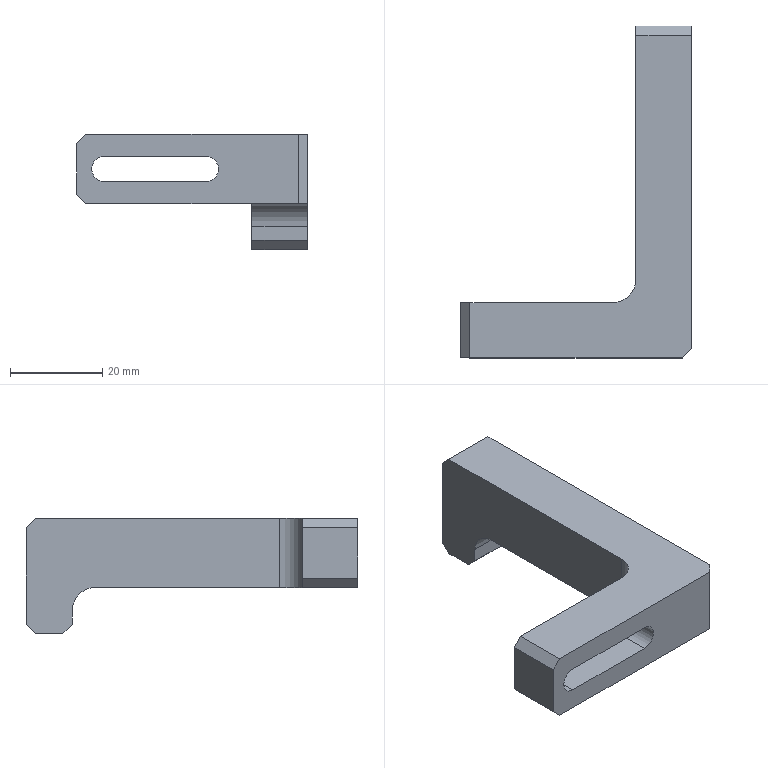Part | NX | 1 solid | 22 faces | box 50 x 72 x 25 mm | volume 19258 mm3 | plane 18 | cylinder 4 | commonest cylinder face diameters 5.5 x2 10 x2
STEP:
#1=CARTESIAN_POINT('',(24.,-33.,-15.));
#2=VERTEX_POINT('',#1);
#3=CARTESIAN_POINT('',(24.,22.,-15.));
#4=VERTEX_POINT('',#3);
#5=CARTESIAN_POINT('',(24.,-35.,-15.));
#6=DIRECTION('',(0.,1.,0.));
#7=VECTOR('',#6,1000.);
#8=LINE('',#5,#7);
#9=EDGE_CURVE('',#2,#4,#8,.T.);
#10=ORIENTED_EDGE('',*,*,#9,.T.);
#11=CARTESIAN_POINT('',(24.,27.,-20.));
#12=VERTEX_POINT('',#11);
#13=CARTESIAN_POINT('',(24.,22.,-20.));
#14=DIRECTION('',(-1.,0.,0.));
#15=DIRECTION('',(0.,0.,-1.));
#16=AXIS2_PLACEMENT_3D('',#13,#14,#15);
#17=CIRCLE('',#16,5.);
#18=EDGE_CURVE('',#4,#12,#17,.T.);
#19=ORIENTED_EDGE('',*,*,#18,.T.);
#20=CARTESIAN_POINT('',(24.,27.,-23.));
#21=VERTEX_POINT('',#20);
#22=CARTESIAN_POINT('',(24.,27.,-15.));
#23=DIRECTION('',(0.,0.,-1.));
#24=VECTOR('',#23,1000.);
#25=LINE('',#22,#24);
#26=EDGE_CURVE('',#12,#21,#25,.T.);
#27=ORIENTED_EDGE('',*,*,#26,.T.);
#28=CARTESIAN_POINT('',(24.,29.,-25.));
#29=VERTEX_POINT('',#28);
#30=CARTESIAN_POINT('',(24.,29.,-25.));
#31=DIRECTION('',(0.,0.7071,-0.7071));
#32=VECTOR('',#31,1000.);
#33=LINE('',#30,#32);
#34=EDGE_CURVE('',#21,#29,#33,.T.);
#35=ORIENTED_EDGE('',*,*,#34,.T.);
#36=CARTESIAN_POINT('',(24.,35.,-25.));
#37=VERTEX_POINT('',#36);
#38=CARTESIAN_POINT('',(24.,-35.,-25.));
#39=DIRECTION('',(0.,1.,0.));
#40=VECTOR('',#39,1000.);
#41=LINE('',#38,#40);
#42=EDGE_CURVE('',#29,#37,#41,.T.);
#43=ORIENTED_EDGE('',*,*,#42,.T.);
#44=CARTESIAN_POINT('',(24.,37.,-23.));
#45=VERTEX_POINT('',#44);
#46=CARTESIAN_POINT('',(24.,35.,-25.));
#47=DIRECTION('',(0.,0.7071,0.7071));
#48=VECTOR('',#47,1000.);
#49=LINE('',#46,#48);
#50=EDGE_CURVE('',#37,#45,#49,.T.);
#51=ORIENTED_EDGE('',*,*,#50,.T.);
#52=CARTESIAN_POINT('',(24.,37.,-2.));
#53=VERTEX_POINT('',#52);
#54=CARTESIAN_POINT('',(24.,37.,-25.));
#55=DIRECTION('',(0.,0.,1.));
#56=VECTOR('',#55,1000.);
#57=LINE('',#54,#56);
#58=EDGE_CURVE('',#45,#53,#57,.T.);
#59=ORIENTED_EDGE('',*,*,#58,.T.);
#60=CARTESIAN_POINT('',(24.,35.,0.));
#61=VERTEX_POINT('',#60);
#62=CARTESIAN_POINT('',(24.,35.,0.));
#63=DIRECTION('',(0.,-0.7071,0.7071));
#64=VECTOR('',#63,1000.);
#65=LINE('',#62,#64);
#66=EDGE_CURVE('',#53,#61,#65,.T.);
#67=ORIENTED_EDGE('',*,*,#66,.T.);
#68=CARTESIAN_POINT('',(24.,-33.,0.));
#69=VERTEX_POINT('',#68);
#70=CARTESIAN_POINT('',(24.,-35.,0.));
#71=DIRECTION('',(0.,1.,0.));
#72=VECTOR('',#71,1000.);
#73=LINE('',#70,#72);
#74=EDGE_CURVE('',#69,#61,#73,.T.);
#75=ORIENTED_EDGE('',*,*,#74,.F.);
#76=CARTESIAN_POINT('',(24.,-33.,-25.));
#77=DIRECTION('',(0.,0.,-1.));
#78=VECTOR('',#77,1000.);
#79=LINE('',#76,#78);
#80=EDGE_CURVE('',#69,#2,#79,.T.);
#81=ORIENTED_EDGE('',*,*,#80,.T.);
#82=EDGE_LOOP('',(#10,#19,#27,#35,#43,#51,#59,#67,#75,#81));
#83=FACE_BOUND('',#82,.T.);
#84=CARTESIAN_POINT('',(24.,-35.,-25.));
#85=DIRECTION('',(-1.,0.,0.));
#86=DIRECTION('',(0.,0.,1.));
#87=AXIS2_PLACEMENT_3D('',#84,#85,#86);
#88=PLANE('',#87);
#89=ADVANCED_FACE('',(#83),#88,.F.);
#90=ORIENTED_EDGE('',*,*,#74,.T.);
#91=CARTESIAN_POINT('',(12.,35.,0.));
#92=VERTEX_POINT('',#91);
#93=CARTESIAN_POINT('',(12.,35.,0.));
#94=DIRECTION('',(-1.,0.,0.));
#95=VECTOR('',#94,1000.);
#96=LINE('',#93,#95);
#97=EDGE_CURVE('',#61,#92,#96,.T.);
#98=ORIENTED_EDGE('',*,*,#97,.T.);
#99=CARTESIAN_POINT('',(12.,-18.,0.));
#100=VERTEX_POINT('',#99);
#101=CARTESIAN_POINT('',(12.,-23.,0.));
#102=DIRECTION('',(0.,1.,0.));
#103=VECTOR('',#102,1000.);
#104=LINE('',#101,#103);
#105=EDGE_CURVE('',#100,#92,#104,.T.);
#106=ORIENTED_EDGE('',*,*,#105,.F.);
#107=CARTESIAN_POINT('',(7.,-23.,0.));
#108=VERTEX_POINT('',#107);
#109=CARTESIAN_POINT('',(7.,-18.,0.));
#110=DIRECTION('',(0.,0.,-1.));
#111=DIRECTION('',(1.,0.,0.));
#112=AXIS2_PLACEMENT_3D('',#109,#110,#111);
#113=CIRCLE('',#112,5.);
#114=EDGE_CURVE('',#100,#108,#113,.T.);
#115=ORIENTED_EDGE('',*,*,#114,.T.);
#116=CARTESIAN_POINT('',(-24.,-23.,0.));
#117=VERTEX_POINT('',#116);
#118=CARTESIAN_POINT('',(-26.,-23.,0.));
#119=DIRECTION('',(1.,0.,0.));
#120=VECTOR('',#119,1000.);
#121=LINE('',#118,#120);
#122=EDGE_CURVE('',#117,#108,#121,.T.);
#123=ORIENTED_EDGE('',*,*,#122,.F.);
#124=CARTESIAN_POINT('',(-24.,-35.,0.));
#125=VERTEX_POINT('',#124);
#126=CARTESIAN_POINT('',(-24.,-35.,0.));
#127=DIRECTION('',(0.,-1.,0.));
#128=VECTOR('',#127,1000.);
#129=LINE('',#126,#128);
#130=EDGE_CURVE('',#117,#125,#129,.T.);
#131=ORIENTED_EDGE('',*,*,#130,.T.);
#132=CARTESIAN_POINT('',(22.,-35.,0.));
#133=VERTEX_POINT('',#132);
#134=CARTESIAN_POINT('',(-26.,-35.,0.));
#135=DIRECTION('',(-1.,0.,0.));
#136=VECTOR('',#135,1000.);
#137=LINE('',#134,#136);
#138=EDGE_CURVE('',#133,#125,#137,.T.);
#139=ORIENTED_EDGE('',*,*,#138,.F.);
#140=CARTESIAN_POINT('',(22.,-35.,0.));
#141=DIRECTION('',(0.7071,0.7071,0.));
#142=VECTOR('',#141,1000.);
#143=LINE('',#140,#142);
#144=EDGE_CURVE('',#133,#69,#143,.T.);
#145=ORIENTED_EDGE('',*,*,#144,.T.);
#146=EDGE_LOOP('',(#90,#98,#106,#115,#123,#131,#139,#145));
#147=FACE_BOUND('',#146,.T.);
#148=CARTESIAN_POINT('',(-26.,-35.,0.));
#149=DIRECTION('',(0.,0.,-1.));
#150=DIRECTION('',(-1.,0.,0.));
#151=AXIS2_PLACEMENT_3D('',#148,#149,#150);
#152=PLANE('',#151);
#153=ADVANCED_FACE('',(#147),#152,.F.);
#154=CARTESIAN_POINT('',(-26.,-35.,-2.));
#155=VERTEX_POINT('',#154);
#156=CARTESIAN_POINT('',(-26.,-35.,-13.));
#157=VERTEX_POINT('',#156);
#158=CARTESIAN_POINT('',(-26.,-35.,-25.));
#159=DIRECTION('',(0.,0.,-1.));
#160=VECTOR('',#159,1000.);
#161=LINE('',#158,#160);
#162=EDGE_CURVE('',#155,#157,#161,.T.);
#163=ORIENTED_EDGE('',*,*,#162,.F.);
#164=CARTESIAN_POINT('',(-26.,-23.,-2.));
#165=VERTEX_POINT('',#164);
#166=CARTESIAN_POINT('',(-26.,-35.,-2.));
#167=DIRECTION('',(0.,1.,0.));
#168=VECTOR('',#167,1000.);
#169=LINE('',#166,#168);
#170=EDGE_CURVE('',#155,#165,#169,.T.);
#171=ORIENTED_EDGE('',*,*,#170,.T.);
#172=CARTESIAN_POINT('',(-26.,-23.,-13.));
#173=VERTEX_POINT('',#172);
#174=CARTESIAN_POINT('',(-26.,-23.,-25.));
#175=DIRECTION('',(0.,0.,1.));
#176=VECTOR('',#175,1000.);
#177=LINE('',#174,#176);
#178=EDGE_CURVE('',#173,#165,#177,.T.);
#179=ORIENTED_EDGE('',*,*,#178,.F.);
#180=CARTESIAN_POINT('',(-26.,-35.,-13.));
#181=DIRECTION('',(0.,-1.,0.));
#182=VECTOR('',#181,1000.);
#183=LINE('',#180,#182);
#184=EDGE_CURVE('',#173,#157,#183,.T.);
#185=ORIENTED_EDGE('',*,*,#184,.T.);
#186=EDGE_LOOP('',(#163,#171,#179,#185));
#187=FACE_BOUND('',#186,.T.);
#188=CARTESIAN_POINT('',(-26.,-35.,-25.));
#189=DIRECTION('',(1.,0.,0.));
#190=DIRECTION('',(0.,1.,0.));
#191=AXIS2_PLACEMENT_3D('',#188,#189,#190);
#192=PLANE('',#191);
#193=ADVANCED_FACE('',(#187),#192,.F.);
#194=ORIENTED_EDGE('',*,*,#42,.F.);
#195=CARTESIAN_POINT('',(12.,29.,-25.));
#196=VERTEX_POINT('',#195);
#197=CARTESIAN_POINT('',(-26.,29.,-25.));
#198=DIRECTION('',(-1.,0.,0.));
#199=VECTOR('',#198,1000.);
#200=LINE('',#197,#199);
#201=EDGE_CURVE('',#29,#196,#200,.T.);
#202=ORIENTED_EDGE('',*,*,#201,.T.);
#203=CARTESIAN_POINT('',(12.,35.,-25.));
#204=VERTEX_POINT('',#203);
#205=CARTESIAN_POINT('',(12.,-23.,-25.));
#206=DIRECTION('',(0.,1.,0.));
#207=VECTOR('',#206,1000.);
#208=LINE('',#205,#207);
#209=EDGE_CURVE('',#196,#204,#208,.T.);
#210=ORIENTED_EDGE('',*,*,#209,.T.);
#211=CARTESIAN_POINT('',(24.,35.,-25.));
#212=DIRECTION('',(1.,0.,0.));
#213=VECTOR('',#212,1000.);
#214=LINE('',#211,#213);
#215=EDGE_CURVE('',#204,#37,#214,.T.);
#216=ORIENTED_EDGE('',*,*,#215,.T.);
#217=EDGE_LOOP('',(#194,#202,#210,#216));
#218=FACE_BOUND('',#217,.T.);
#219=CARTESIAN_POINT('',(-26.,-35.,-25.));
#220=DIRECTION('',(0.,0.,1.));
#221=DIRECTION('',(1.,0.,0.));
#222=AXIS2_PLACEMENT_3D('',#219,#220,#221);
#223=PLANE('',#222);
#224=ADVANCED_FACE('',(#218),#223,.F.);
#225=CARTESIAN_POINT('',(-20.,-35.,-4.75));
#226=VERTEX_POINT('',#225);
#227=CARTESIAN_POINT('',(2.,-35.,-4.75));
#228=VERTEX_POINT('',#227);
#229=CARTESIAN_POINT('',(-20.,-35.,-4.75));
#230=DIRECTION('',(1.,0.,0.));
#231=VECTOR('',#230,1000.);
#232=LINE('',#229,#231);
#233=EDGE_CURVE('',#226,#228,#232,.T.);
#234=ORIENTED_EDGE('',*,*,#233,.T.);
#235=CARTESIAN_POINT('',(2.,-35.,-10.25));
#236=VERTEX_POINT('',#235);
#237=CARTESIAN_POINT('',(2.,-35.,-7.5));
#238=DIRECTION('',(0.,1.,0.));
#239=DIRECTION('',(0.,0.,-1.));
#240=AXIS2_PLACEMENT_3D('',#237,#238,#239);
#241=CIRCLE('',#240,2.75);
#242=EDGE_CURVE('',#228,#236,#241,.T.);
#243=ORIENTED_EDGE('',*,*,#242,.T.);
#244=CARTESIAN_POINT('',(-20.,-35.,-10.25));
#245=VERTEX_POINT('',#244);
#246=CARTESIAN_POINT('',(-20.,-35.,-10.25));
#247=DIRECTION('',(1.,0.,0.));
#248=VECTOR('',#247,1000.);
#249=LINE('',#246,#248);
#250=EDGE_CURVE('',#245,#236,#249,.T.);
#251=ORIENTED_EDGE('',*,*,#250,.F.);
#252=CARTESIAN_POINT('',(-20.,-35.,-7.5));
#253=DIRECTION('',(0.,1.,0.));
#254=DIRECTION('',(0.,0.,-1.));
#255=AXIS2_PLACEMENT_3D('',#252,#253,#254);
#256=CIRCLE('',#255,2.75);
#257=EDGE_CURVE('',#245,#226,#256,.T.);
#258=ORIENTED_EDGE('',*,*,#257,.T.);
#259=EDGE_LOOP('',(#234,#243,#251,#258));
#260=FACE_BOUND('',#259,.T.);
#261=CARTESIAN_POINT('',(22.,-35.,-15.));
#262=VERTEX_POINT('',#261);
#263=CARTESIAN_POINT('',(-24.,-35.,-15.));
#264=VERTEX_POINT('',#263);
#265=CARTESIAN_POINT('',(24.,-35.,-15.));
#266=DIRECTION('',(-1.,0.,0.));
#267=VECTOR('',#266,1000.);
#268=LINE('',#265,#267);
#269=EDGE_CURVE('',#262,#264,#268,.T.);
#270=ORIENTED_EDGE('',*,*,#269,.F.);
#271=CARTESIAN_POINT('',(22.,-35.,-12.5));
#272=DIRECTION('',(0.,0.,1.));
#273=VECTOR('',#272,1000.);
#274=LINE('',#271,#273);
#275=EDGE_CURVE('',#262,#133,#274,.T.);
#276=ORIENTED_EDGE('',*,*,#275,.T.);
#277=ORIENTED_EDGE('',*,*,#138,.T.);
#278=CARTESIAN_POINT('',(-26.,-35.,-2.));
#279=DIRECTION('',(-0.7071,0.,-0.7071));
#280=VECTOR('',#279,1000.);
#281=LINE('',#278,#280);
#282=EDGE_CURVE('',#125,#155,#281,.T.);
#283=ORIENTED_EDGE('',*,*,#282,.T.);
#284=ORIENTED_EDGE('',*,*,#162,.T.);
#285=CARTESIAN_POINT('',(-24.,-35.,-15.));
#286=DIRECTION('',(0.7071,0.,-0.7071));
#287=VECTOR('',#286,1000.);
#288=LINE('',#285,#287);
#289=EDGE_CURVE('',#157,#264,#288,.T.);
#290=ORIENTED_EDGE('',*,*,#289,.T.);
#291=EDGE_LOOP('',(#270,#276,#277,#283,#284,#290));
#292=FACE_BOUND('',#291,.T.);
#293=CARTESIAN_POINT('',(-1.,-35.,-12.5));
#294=DIRECTION('',(0.,1.,0.));
#295=DIRECTION('',(-1.,0.,0.));
#296=AXIS2_PLACEMENT_3D('',#293,#294,#295);
#297=PLANE('',#296);
#298=ADVANCED_FACE('',(#260,#292),#297,.F.);
#299=ORIENTED_EDGE('',*,*,#58,.F.);
#300=CARTESIAN_POINT('',(12.,37.,-23.));
#301=VERTEX_POINT('',#300);
#302=CARTESIAN_POINT('',(12.,37.,-23.));
#303=DIRECTION('',(-1.,0.,0.));
#304=VECTOR('',#303,1000.);
#305=LINE('',#302,#304);
#306=EDGE_CURVE('',#45,#301,#305,.T.);
#307=ORIENTED_EDGE('',*,*,#306,.T.);
#308=CARTESIAN_POINT('',(12.,37.,-2.));
#309=VERTEX_POINT('',#308);
#310=CARTESIAN_POINT('',(12.,37.,-25.));
#311=DIRECTION('',(0.,0.,1.));
#312=VECTOR('',#311,1000.);
#313=LINE('',#310,#312);
#314=EDGE_CURVE('',#301,#309,#313,.T.);
#315=ORIENTED_EDGE('',*,*,#314,.T.);
#316=CARTESIAN_POINT('',(24.,37.,-2.));
#317=DIRECTION('',(1.,0.,0.));
#318=VECTOR('',#317,1000.);
#319=LINE('',#316,#318);
#320=EDGE_CURVE('',#309,#53,#319,.T.);
#321=ORIENTED_EDGE('',*,*,#320,.T.);
#322=EDGE_LOOP('',(#299,#307,#315,#321));
#323=FACE_BOUND('',#322,.T.);
#324=CARTESIAN_POINT('',(-1.,37.,-12.5));
#325=DIRECTION('',(0.,1.,0.));
#326=DIRECTION('',(-1.,0.,0.));
#327=AXIS2_PLACEMENT_3D('',#324,#325,#326);
#328=PLANE('',#327);
#329=ADVANCED_FACE('',(#323),#328,.T.);
#330=ORIENTED_EDGE('',*,*,#209,.F.);
#331=CARTESIAN_POINT('',(12.,27.,-23.));
#332=VERTEX_POINT('',#331);
#333=CARTESIAN_POINT('',(12.,29.,-25.));
#334=DIRECTION('',(0.,-0.7071,0.7071));
#335=VECTOR('',#334,1000.);
#336=LINE('',#333,#335);
#337=EDGE_CURVE('',#196,#332,#336,.T.);
#338=ORIENTED_EDGE('',*,*,#337,.T.);
#339=CARTESIAN_POINT('',(12.,27.,-20.));
#340=VERTEX_POINT('',#339);
#341=CARTESIAN_POINT('',(12.,27.,-25.));
#342=DIRECTION('',(0.,0.,1.));
#343=VECTOR('',#342,1000.);
#344=LINE('',#341,#343);
#345=EDGE_CURVE('',#332,#340,#344,.T.);
#346=ORIENTED_EDGE('',*,*,#345,.T.);
#347=CARTESIAN_POINT('',(12.,22.,-15.));
#348=VERTEX_POINT('',#347);
#349=CARTESIAN_POINT('',(12.,22.,-20.));
#350=DIRECTION('',(1.,0.,0.));
#351=DIRECTION('',(0.,-1.,0.));
#352=AXIS2_PLACEMENT_3D('',#349,#350,#351);
#353=CIRCLE('',#352,5.);
#354=EDGE_CURVE('',#340,#348,#353,.T.);
#355=ORIENTED_EDGE('',*,*,#354,.T.);
#356=CARTESIAN_POINT('',(12.,-18.,-15.));
#357=VERTEX_POINT('',#356);
#358=CARTESIAN_POINT('',(12.,-23.,-15.));
#359=DIRECTION('',(0.,-1.,0.));
#360=VECTOR('',#359,1000.);
#361=LINE('',#358,#360);
#362=EDGE_CURVE('',#348,#357,#361,.T.);
#363=ORIENTED_EDGE('',*,*,#362,.T.);
#364=CARTESIAN_POINT('',(12.,-18.,0.));
#365=DIRECTION('',(0.,0.,1.));
#366=VECTOR('',#365,1000.);
#367=LINE('',#364,#366);
#368=EDGE_CURVE('',#357,#100,#367,.T.);
#369=ORIENTED_EDGE('',*,*,#368,.T.);
#370=ORIENTED_EDGE('',*,*,#105,.T.);
#371=CARTESIAN_POINT('',(12.,35.,0.));
#372=DIRECTION('',(0.,0.7071,-0.7071));
#373=VECTOR('',#372,1000.);
#374=LINE('',#371,#373);
#375=EDGE_CURVE('',#92,#309,#374,.T.);
#376=ORIENTED_EDGE('',*,*,#375,.T.);
#377=ORIENTED_EDGE('',*,*,#314,.F.);
#378=CARTESIAN_POINT('',(12.,35.,-25.));
#379=DIRECTION('',(0.,-0.7071,-0.7071));
#380=VECTOR('',#379,1000.);
#381=LINE('',#378,#380);
#382=EDGE_CURVE('',#301,#204,#381,.T.);
#383=ORIENTED_EDGE('',*,*,#382,.T.);
#384=EDGE_LOOP('',(#330,#338,#346,#355,#363,#369,#370,#376,#377,#383));
#385=FACE_BOUND('',#384,.T.);
#386=CARTESIAN_POINT('',(12.,-23.,-25.));
#387=DIRECTION('',(1.,0.,0.));
#388=DIRECTION('',(0.,1.,0.));
#389=AXIS2_PLACEMENT_3D('',#386,#387,#388);
#390=PLANE('',#389);
#391=ADVANCED_FACE('',(#385),#390,.F.);
#392=CARTESIAN_POINT('',(-20.,-23.,-4.75));
#393=VERTEX_POINT('',#392);
#394=CARTESIAN_POINT('',(2.,-23.,-4.75));
#395=VERTEX_POINT('',#394);
#396=CARTESIAN_POINT('',(-20.,-23.,-4.75));
#397=DIRECTION('',(1.,0.,0.));
#398=VECTOR('',#397,1000.);
#399=LINE('',#396,#398);
#400=EDGE_CURVE('',#393,#395,#399,.T.);
#401=ORIENTED_EDGE('',*,*,#400,.F.);
#402=CARTESIAN_POINT('',(-20.,-23.,-10.25));
#403=VERTEX_POINT('',#402);
#404=CARTESIAN_POINT('',(-20.,-23.,-7.5));
#405=DIRECTION('',(0.,1.,0.));
#406=DIRECTION('',(0.,0.,-1.));
#407=AXIS2_PLACEMENT_3D('',#404,#405,#406);
#408=CIRCLE('',#407,2.75);
#409=EDGE_CURVE('',#403,#393,#408,.T.);
#410=ORIENTED_EDGE('',*,*,#409,.F.);
#411=CARTESIAN_POINT('',(2.,-23.,-10.25));
#412=VERTEX_POINT('',#411);
#413=CARTESIAN_POINT('',(-20.,-23.,-10.25));
#414=DIRECTION('',(1.,0.,0.));
#415=VECTOR('',#414,1000.);
#416=LINE('',#413,#415);
#417=EDGE_CURVE('',#403,#412,#416,.T.);
#418=ORIENTED_EDGE('',*,*,#417,.T.);
#419=CARTESIAN_POINT('',(2.,-23.,-7.5));
#420=DIRECTION('',(0.,1.,0.));
#421=DIRECTION('',(0.,0.,-1.));
#422=AXIS2_PLACEMENT_3D('',#419,#420,#421);
#423=CIRCLE('',#422,2.75);
#424=EDGE_CURVE('',#395,#412,#423,.T.);
#425=ORIENTED_EDGE('',*,*,#424,.F.);
#426=EDGE_LOOP('',(#401,#410,#418,#425));
#427=FACE_BOUND('',#426,.T.);
#428=ORIENTED_EDGE('',*,*,#178,.T.);
#429=CARTESIAN_POINT('',(-26.,-23.,-2.));
#430=DIRECTION('',(0.7071,0.,0.7071));
#431=VECTOR('',#430,1000.);
#432=LINE('',#429,#431);
#433=EDGE_CURVE('',#165,#117,#432,.T.);
#434=ORIENTED_EDGE('',*,*,#433,.T.);
#435=ORIENTED_EDGE('',*,*,#122,.T.);
#436=CARTESIAN_POINT('',(7.,-23.,-15.));
#437=VERTEX_POINT('',#436);
#438=CARTESIAN_POINT('',(7.,-23.,-15.));
#439=DIRECTION('',(0.,0.,-1.));
#440=VECTOR('',#439,1000.);
#441=LINE('',#438,#440);
#442=EDGE_CURVE('',#108,#437,#441,.T.);
#443=ORIENTED_EDGE('',*,*,#442,.T.);
#444=CARTESIAN_POINT('',(-24.,-23.,-15.));
#445=VERTEX_POINT('',#444);
#446=CARTESIAN_POINT('',(-26.,-23.,-15.));
#447=DIRECTION('',(-1.,0.,0.));
#448=VECTOR('',#447,1000.);
#449=LINE('',#446,#448);
#450=EDGE_CURVE('',#437,#445,#449,.T.);
#451=ORIENTED_EDGE('',*,*,#450,.T.);
#452=CARTESIAN_POINT('',(-24.,-23.,-15.));
#453=DIRECTION('',(-0.7071,0.,0.7071));
#454=VECTOR('',#453,1000.);
#455=LINE('',#452,#454);
#456=EDGE_CURVE('',#445,#173,#455,.T.);
#457=ORIENTED_EDGE('',*,*,#456,.T.);
#458=EDGE_LOOP('',(#428,#434,#435,#443,#451,#457));
#459=FACE_BOUND('',#458,.T.);
#460=CARTESIAN_POINT('',(-26.,-23.,-25.));
#461=DIRECTION('',(0.,-1.,0.));
#462=DIRECTION('',(1.,0.,0.));
#463=AXIS2_PLACEMENT_3D('',#460,#461,#462);
#464=PLANE('',#463);
#465=ADVANCED_FACE('',(#427,#459),#464,.F.);
#466=ORIENTED_EDGE('',*,*,#26,.F.);
#467=CARTESIAN_POINT('',(12.,27.,-20.));
#468=DIRECTION('',(-1.,0.,0.));
#469=VECTOR('',#468,1000.);
#470=LINE('',#467,#469);
#471=EDGE_CURVE('',#12,#340,#470,.T.);
#472=ORIENTED_EDGE('',*,*,#471,.T.);
#473=ORIENTED_EDGE('',*,*,#345,.F.);
#474=CARTESIAN_POINT('',(24.,27.,-23.));
#475=DIRECTION('',(1.,0.,0.));
#476=VECTOR('',#475,1000.);
#477=LINE('',#474,#476);
#478=EDGE_CURVE('',#332,#21,#477,.T.);
#479=ORIENTED_EDGE('',*,*,#478,.T.);
#480=EDGE_LOOP('',(#466,#472,#473,#479));
#481=FACE_BOUND('',#480,.T.);
#482=CARTESIAN_POINT('',(24.,27.,-15.));
#483=DIRECTION('',(0.,1.,0.));
#484=DIRECTION('',(-1.,0.,0.));
#485=AXIS2_PLACEMENT_3D('',#482,#483,#484);
#486=PLANE('',#485);
#487=ADVANCED_FACE('',(#481),#486,.F.);
#488=ORIENTED_EDGE('',*,*,#362,.F.);
#489=CARTESIAN_POINT('',(24.,22.,-15.));
#490=DIRECTION('',(1.,0.,0.));
#491=VECTOR('',#490,1000.);
#492=LINE('',#489,#491);
#493=EDGE_CURVE('',#348,#4,#492,.T.);
#494=ORIENTED_EDGE('',*,*,#493,.T.);
#495=ORIENTED_EDGE('',*,*,#9,.F.);
#496=CARTESIAN_POINT('',(22.,-35.,-15.));
#497=DIRECTION('',(-0.7071,-0.7071,0.));
#498=VECTOR('',#497,1000.);
#499=LINE('',#496,#498);
#500=EDGE_CURVE('',#2,#262,#499,.T.);
#501=ORIENTED_EDGE('',*,*,#500,.T.);
#502=ORIENTED_EDGE('',*,*,#269,.T.);
#503=CARTESIAN_POINT('',(-24.,-35.,-15.));
#504=DIRECTION('',(0.,1.,0.));
#505=VECTOR('',#504,1000.);
#506=LINE('',#503,#505);
#507=EDGE_CURVE('',#264,#445,#506,.T.);
#508=ORIENTED_EDGE('',*,*,#507,.T.);
#509=ORIENTED_EDGE('',*,*,#450,.F.);
#510=CARTESIAN_POINT('',(7.,-18.,-15.));
#511=DIRECTION('',(0.,0.,1.));
#512=DIRECTION('',(0.,1.,0.));
#513=AXIS2_PLACEMENT_3D('',#510,#511,#512);
#514=CIRCLE('',#513,5.);
#515=EDGE_CURVE('',#437,#357,#514,.T.);
#516=ORIENTED_EDGE('',*,*,#515,.T.);
#517=EDGE_LOOP('',(#488,#494,#495,#501,#502,#508,#509,#516));
#518=FACE_BOUND('',#517,.T.);
#519=CARTESIAN_POINT('',(24.,-35.,-15.));
#520=DIRECTION('',(0.,0.,1.));
#521=DIRECTION('',(0.,-1.,0.));
#522=AXIS2_PLACEMENT_3D('',#519,#520,#521);
#523=PLANE('',#522);
#524=ADVANCED_FACE('',(#518),#523,.F.);
#525=ORIENTED_EDGE('',*,*,#515,.F.);
#526=ORIENTED_EDGE('',*,*,#442,.F.);
#527=ORIENTED_EDGE('',*,*,#114,.F.);
#528=ORIENTED_EDGE('',*,*,#368,.F.);
#529=EDGE_LOOP('',(#525,#526,#527,#528));
#530=FACE_BOUND('',#529,.T.);
#531=CARTESIAN_POINT('',(7.,-18.,-25.));
#532=DIRECTION('',(0.,0.,-1.));
#533=DIRECTION('',(-1.,0.,0.));
#534=AXIS2_PLACEMENT_3D('',#531,#532,#533);
#535=CYLINDRICAL_SURFACE('',#534,5.);
#536=ADVANCED_FACE('',(#530),#535,.F.);
#537=ORIENTED_EDGE('',*,*,#424,.T.);
#538=CARTESIAN_POINT('',(2.,-23.,-10.25));
#539=DIRECTION('',(0.,1.,0.));
#540=VECTOR('',#539,1000.);
#541=LINE('',#538,#540);
#542=EDGE_CURVE('',#236,#412,#541,.T.);
#543=ORIENTED_EDGE('',*,*,#542,.F.);
#544=ORIENTED_EDGE('',*,*,#242,.F.);
#545=CARTESIAN_POINT('',(2.,-23.,-4.75));
#546=DIRECTION('',(0.,-1.,0.));
#547=VECTOR('',#546,1000.);
#548=LINE('',#545,#547);
#549=EDGE_CURVE('',#395,#228,#548,.T.);
#550=ORIENTED_EDGE('',*,*,#549,.F.);
#551=EDGE_LOOP('',(#537,#543,#544,#550));
#552=FACE_BOUND('',#551,.T.);
#553=CARTESIAN_POINT('',(2.,-23.,-7.5));
#554=DIRECTION('',(0.,1.,0.));
#555=DIRECTION('',(0.,0.,1.));
#556=AXIS2_PLACEMENT_3D('',#553,#554,#555);
#557=CYLINDRICAL_SURFACE('',#556,2.75);
#558=ADVANCED_FACE('',(#552),#557,.F.);
#559=ORIENTED_EDGE('',*,*,#409,.T.);
#560=CARTESIAN_POINT('',(-20.,-23.,-4.75));
#561=DIRECTION('',(0.,1.,0.));
#562=VECTOR('',#561,1000.);
#563=LINE('',#560,#562);
#564=EDGE_CURVE('',#226,#393,#563,.T.);
#565=ORIENTED_EDGE('',*,*,#564,.F.);
#566=ORIENTED_EDGE('',*,*,#257,.F.);
#567=CARTESIAN_POINT('',(-20.,-23.,-10.25));
#568=DIRECTION('',(0.,-1.,0.));
#569=VECTOR('',#568,1000.);
#570=LINE('',#567,#569);
#571=EDGE_CURVE('',#403,#245,#570,.T.);
#572=ORIENTED_EDGE('',*,*,#571,.F.);
#573=EDGE_LOOP('',(#559,#565,#566,#572));
#574=FACE_BOUND('',#573,.T.);
#575=CARTESIAN_POINT('',(-20.,-23.,-7.5));
#576=DIRECTION('',(0.,1.,0.));
#577=DIRECTION('',(0.,0.,1.));
#578=AXIS2_PLACEMENT_3D('',#575,#576,#577);
#579=CYLINDRICAL_SURFACE('',#578,2.75);
#580=ADVANCED_FACE('',(#574),#579,.F.);
#581=ORIENTED_EDGE('',*,*,#542,.T.);
#582=ORIENTED_EDGE('',*,*,#417,.F.);
#583=ORIENTED_EDGE('',*,*,#571,.T.);
#584=ORIENTED_EDGE('',*,*,#250,.T.);
#585=EDGE_LOOP('',(#581,#582,#583,#584));
#586=FACE_BOUND('',#585,.T.);
#587=CARTESIAN_POINT('',(-20.,-23.,-10.25));
#588=DIRECTION('',(0.,0.,-1.));
#589=DIRECTION('',(-1.,0.,0.));
#590=AXIS2_PLACEMENT_3D('',#587,#588,#589);
#591=PLANE('',#590);
#592=ADVANCED_FACE('',(#586),#591,.F.);
#593=ORIENTED_EDGE('',*,*,#549,.T.);
#594=ORIENTED_EDGE('',*,*,#233,.F.);
#595=ORIENTED_EDGE('',*,*,#564,.T.);
#596=ORIENTED_EDGE('',*,*,#400,.T.);
#597=EDGE_LOOP('',(#593,#594,#595,#596));
#598=FACE_BOUND('',#597,.T.);
#599=CARTESIAN_POINT('',(-20.,-23.,-4.75));
#600=DIRECTION('',(0.,0.,1.));
#601=DIRECTION('',(1.,0.,0.));
#602=AXIS2_PLACEMENT_3D('',#599,#600,#601);
#603=PLANE('',#602);
#604=ADVANCED_FACE('',(#598),#603,.F.);
#605=ORIENTED_EDGE('',*,*,#34,.F.);
#606=ORIENTED_EDGE('',*,*,#478,.F.);
#607=ORIENTED_EDGE('',*,*,#337,.F.);
#608=ORIENTED_EDGE('',*,*,#201,.F.);
#609=EDGE_LOOP('',(#605,#606,#607,#608));
#610=FACE_BOUND('',#609,.T.);
#611=CARTESIAN_POINT('',(-26.,29.,-25.));
#612=DIRECTION('',(0.,0.7071,0.7071));
#613=DIRECTION('',(1.,0.,0.));
#614=AXIS2_PLACEMENT_3D('',#611,#612,#613);
#615=PLANE('',#614);
#616=ADVANCED_FACE('',(#610),#615,.F.);
#617=ORIENTED_EDGE('',*,*,#382,.F.);
#618=ORIENTED_EDGE('',*,*,#306,.F.);
#619=ORIENTED_EDGE('',*,*,#50,.F.);
#620=ORIENTED_EDGE('',*,*,#215,.F.);
#621=EDGE_LOOP('',(#617,#618,#619,#620));
#622=FACE_BOUND('',#621,.T.);
#623=CARTESIAN_POINT('',(-26.,35.,-25.));
#624=DIRECTION('',(0.,0.7071,-0.7071));
#625=DIRECTION('',(1.,0.,0.));
#626=AXIS2_PLACEMENT_3D('',#623,#624,#625);
#627=PLANE('',#626);
#628=ADVANCED_FACE('',(#622),#627,.T.);
#629=ORIENTED_EDGE('',*,*,#66,.F.);
#630=ORIENTED_EDGE('',*,*,#320,.F.);
#631=ORIENTED_EDGE('',*,*,#375,.F.);
#632=ORIENTED_EDGE('',*,*,#97,.F.);
#633=EDGE_LOOP('',(#629,#630,#631,#632));
#634=FACE_BOUND('',#633,.T.);
#635=CARTESIAN_POINT('',(-26.,35.,0.));
#636=DIRECTION('',(0.,0.7071,0.7071));
#637=DIRECTION('',(-1.,0.,0.));
#638=AXIS2_PLACEMENT_3D('',#635,#636,#637);
#639=PLANE('',#638);
#640=ADVANCED_FACE('',(#634),#639,.T.);
#641=ORIENTED_EDGE('',*,*,#500,.F.);
#642=ORIENTED_EDGE('',*,*,#80,.F.);
#643=ORIENTED_EDGE('',*,*,#144,.F.);
#644=ORIENTED_EDGE('',*,*,#275,.F.);
#645=EDGE_LOOP('',(#641,#642,#643,#644));
#646=FACE_BOUND('',#645,.T.);
#647=CARTESIAN_POINT('',(22.,-35.,-12.5));
#648=DIRECTION('',(-0.7071,0.7071,0.));
#649=DIRECTION('',(0.,0.,-1.));
#650=AXIS2_PLACEMENT_3D('',#647,#648,#649);
#651=PLANE('',#650);
#652=ADVANCED_FACE('',(#646),#651,.F.);
#653=ORIENTED_EDGE('',*,*,#282,.F.);
#654=ORIENTED_EDGE('',*,*,#130,.F.);
#655=ORIENTED_EDGE('',*,*,#433,.F.);
#656=ORIENTED_EDGE('',*,*,#170,.F.);
#657=EDGE_LOOP('',(#653,#654,#655,#656));
#658=FACE_BOUND('',#657,.T.);
#659=CARTESIAN_POINT('',(-26.,-35.,-2.));
#660=DIRECTION('',(0.7071,0.,-0.7071));
#661=DIRECTION('',(0.,-1.,0.));
#662=AXIS2_PLACEMENT_3D('',#659,#660,#661);
#663=PLANE('',#662);
#664=ADVANCED_FACE('',(#658),#663,.F.);
#665=ORIENTED_EDGE('',*,*,#289,.F.);
#666=ORIENTED_EDGE('',*,*,#184,.F.);
#667=ORIENTED_EDGE('',*,*,#456,.F.);
#668=ORIENTED_EDGE('',*,*,#507,.F.);
#669=EDGE_LOOP('',(#665,#666,#667,#668));
#670=FACE_BOUND('',#669,.T.);
#671=CARTESIAN_POINT('',(-24.,-35.,-15.));
#672=DIRECTION('',(0.7071,0.,0.7071));
#673=DIRECTION('',(0.,-1.,0.));
#674=AXIS2_PLACEMENT_3D('',#671,#672,#673);
#675=PLANE('',#674);
#676=ADVANCED_FACE('',(#670),#675,.F.);
#677=ORIENTED_EDGE('',*,*,#18,.F.);
#678=ORIENTED_EDGE('',*,*,#493,.F.);
#679=ORIENTED_EDGE('',*,*,#354,.F.);
#680=ORIENTED_EDGE('',*,*,#471,.F.);
#681=EDGE_LOOP('',(#677,#678,#679,#680));
#682=FACE_BOUND('',#681,.T.);
#683=CARTESIAN_POINT('',(24.,22.,-20.));
#684=DIRECTION('',(1.,0.,0.));
#685=DIRECTION('',(0.,1.,0.));
#686=AXIS2_PLACEMENT_3D('',#683,#684,#685);
#687=CYLINDRICAL_SURFACE('',#686,5.);
#688=ADVANCED_FACE('',(#682),#687,.F.);
#689=CLOSED_SHELL('',(#89,#153,#193,#224,#298,#329,#391,#465,#487,#524,#536,#558,#580,#592,#604,#616,#628,#640,#652,#664,#676,#688));
#690=MANIFOLD_SOLID_BREP('',#689);
#691=(LENGTH_UNIT()NAMED_UNIT(*)SI_UNIT(.MILLI.,.METRE.));
#692=UNCERTAINTY_MEASURE_WITH_UNIT(LENGTH_MEASURE(0.00001),#691,'','');
#693=(NAMED_UNIT(*)PLANE_ANGLE_UNIT()SI_UNIT($,.RADIAN.));
#694=(NAMED_UNIT(*)SI_UNIT($,.STERADIAN.)SOLID_ANGLE_UNIT());
#695=(GEOMETRIC_REPRESENTATION_CONTEXT(3)GLOBAL_UNCERTAINTY_ASSIGNED_CONTEXT((#692))GLOBAL_UNIT_ASSIGNED_CONTEXT((#691,#693,#694))REPRESENTATION_CONTEXT('',''));
#696=ADVANCED_BREP_SHAPE_REPRESENTATION('',(#690),#695);